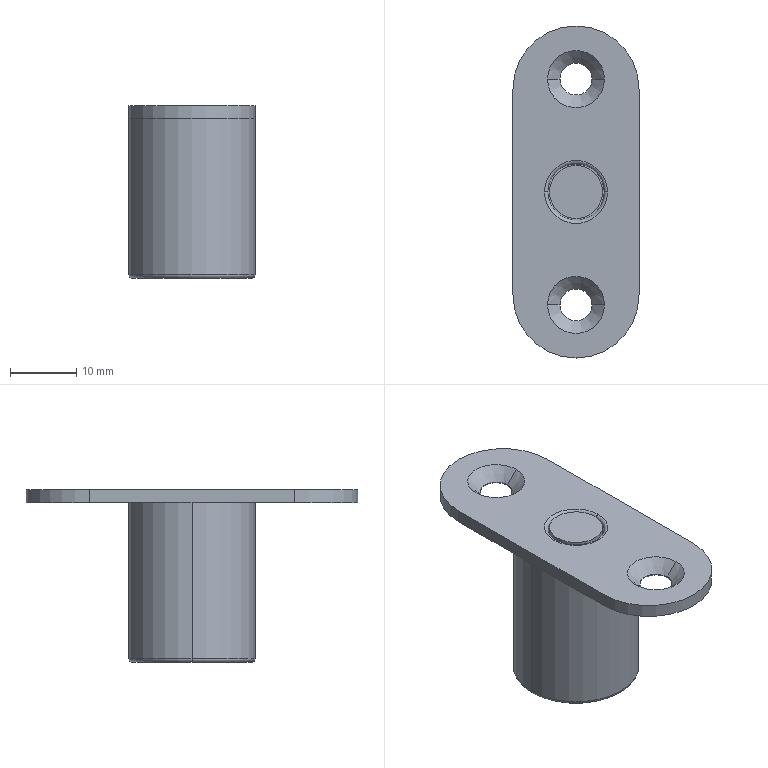Part | NX | features BREP 1 | 1 solid | 33 faces | box 19 x 50 x 26 mm | volume 8272 mm3 | plane 13 | cylinder 12 | cone 4 | torus 4 | commonest cylinder face diameters 4.8 x4 19 x4 8 x2 8.5 x2
STEP:
#1=CARTESIAN_POINT('',(-2.4,17.,-1.9));
#2=VERTEX_POINT('',#1);
#3=CARTESIAN_POINT('',(2.4,17.,-1.9));
#4=VERTEX_POINT('',#3);
#5=CARTESIAN_POINT('',(0.,17.,-1.9));
#6=DIRECTION('',(0.,0.,1.));
#7=DIRECTION('',(1.,0.,0.));
#8=AXIS2_PLACEMENT_3D('',#5,#6,#7);
#9=CIRCLE('',#8,2.4);
#10=EDGE_CURVE('',#2,#4,#9,.T.);
#11=ORIENTED_EDGE('',*,*,#10,.F.);
#12=CARTESIAN_POINT('',(-4.3,17.,0.));
#13=VERTEX_POINT('',#12);
#14=CARTESIAN_POINT('',(-2.4,17.,-1.9));
#15=DIRECTION('',(-0.7071,0.,0.7071));
#16=VECTOR('',#15,1000.);
#17=LINE('',#14,#16);
#18=EDGE_CURVE('',#13,#2,#17,.F.);
#19=ORIENTED_EDGE('',*,*,#18,.F.);
#20=CARTESIAN_POINT('',(4.3,17.,0.));
#21=VERTEX_POINT('',#20);
#22=CARTESIAN_POINT('',(0.,17.,0.));
#23=DIRECTION('',(0.,0.,-1.));
#24=DIRECTION('',(1.,0.,0.));
#25=AXIS2_PLACEMENT_3D('',#22,#23,#24);
#26=CIRCLE('',#25,4.3);
#27=EDGE_CURVE('',#21,#13,#26,.T.);
#28=ORIENTED_EDGE('',*,*,#27,.F.);
#29=CARTESIAN_POINT('',(2.4,17.,-1.9));
#30=DIRECTION('',(0.7071,0.,0.7071));
#31=VECTOR('',#30,1000.);
#32=LINE('',#29,#31);
#33=EDGE_CURVE('',#21,#4,#32,.F.);
#34=ORIENTED_EDGE('',*,*,#33,.T.);
#35=EDGE_LOOP('',(#11,#19,#28,#34));
#36=FACE_BOUND('',#35,.T.);
#37=CARTESIAN_POINT('',(0.,17.,-1.9));
#38=DIRECTION('',(0.,0.,1.));
#39=DIRECTION('',(1.,0.,0.));
#40=AXIS2_PLACEMENT_3D('',#37,#38,#39);
#41=CONICAL_SURFACE('',#40,2.4,0.7854);
#42=ADVANCED_FACE('',(#36),#41,.F.);
#43=CARTESIAN_POINT('',(-2.4,-17.,-1.9));
#44=VERTEX_POINT('',#43);
#45=CARTESIAN_POINT('',(2.4,-17.,-1.9));
#46=VERTEX_POINT('',#45);
#47=CARTESIAN_POINT('',(0.,-17.,-1.9));
#48=DIRECTION('',(0.,0.,1.));
#49=DIRECTION('',(1.,0.,0.));
#50=AXIS2_PLACEMENT_3D('',#47,#48,#49);
#51=CIRCLE('',#50,2.4);
#52=EDGE_CURVE('',#44,#46,#51,.T.);
#53=ORIENTED_EDGE('',*,*,#52,.F.);
#54=CARTESIAN_POINT('',(-4.3,-17.,0.));
#55=VERTEX_POINT('',#54);
#56=CARTESIAN_POINT('',(-2.4,-17.,-1.9));
#57=DIRECTION('',(-0.7071,0.,0.7071));
#58=VECTOR('',#57,1000.);
#59=LINE('',#56,#58);
#60=EDGE_CURVE('',#55,#44,#59,.F.);
#61=ORIENTED_EDGE('',*,*,#60,.F.);
#62=CARTESIAN_POINT('',(4.3,-17.,0.));
#63=VERTEX_POINT('',#62);
#64=CARTESIAN_POINT('',(0.,-17.,0.));
#65=DIRECTION('',(0.,0.,-1.));
#66=DIRECTION('',(1.,0.,0.));
#67=AXIS2_PLACEMENT_3D('',#64,#65,#66);
#68=CIRCLE('',#67,4.3);
#69=EDGE_CURVE('',#63,#55,#68,.T.);
#70=ORIENTED_EDGE('',*,*,#69,.F.);
#71=CARTESIAN_POINT('',(2.4,-17.,-1.9));
#72=DIRECTION('',(0.7071,0.,0.7071));
#73=VECTOR('',#72,1000.);
#74=LINE('',#71,#73);
#75=EDGE_CURVE('',#63,#46,#74,.F.);
#76=ORIENTED_EDGE('',*,*,#75,.T.);
#77=EDGE_LOOP('',(#53,#61,#70,#76));
#78=FACE_BOUND('',#77,.T.);
#79=CARTESIAN_POINT('',(0.,-17.,-1.9));
#80=DIRECTION('',(0.,0.,1.));
#81=DIRECTION('',(1.,0.,0.));
#82=AXIS2_PLACEMENT_3D('',#79,#80,#81);
#83=CONICAL_SURFACE('',#82,2.4,0.7854);
#84=ADVANCED_FACE('',(#78),#83,.F.);
#85=CARTESIAN_POINT('',(-4.75,0.,0.));
#86=VERTEX_POINT('',#85);
#87=CARTESIAN_POINT('',(4.75,0.,0.));
#88=VERTEX_POINT('',#87);
#89=CARTESIAN_POINT('',(0.,0.,0.));
#90=DIRECTION('',(0.,0.,-1.));
#91=DIRECTION('',(1.,0.,0.));
#92=AXIS2_PLACEMENT_3D('',#89,#90,#91);
#93=CIRCLE('',#92,4.75);
#94=EDGE_CURVE('',#86,#88,#93,.T.);
#95=ORIENTED_EDGE('',*,*,#94,.F.);
#96=CARTESIAN_POINT('',(-4.25,0.,-0.5));
#97=VERTEX_POINT('',#96);
#98=CARTESIAN_POINT('',(-4.75,0.,-0.5));
#99=DIRECTION('',(0.,1.,0.));
#100=DIRECTION('',(-1.,0.,0.));
#101=AXIS2_PLACEMENT_3D('',#98,#99,#100);
#102=CIRCLE('',#101,0.5);
#103=EDGE_CURVE('',#97,#86,#102,.F.);
#104=ORIENTED_EDGE('',*,*,#103,.F.);
#105=CARTESIAN_POINT('',(4.25,0.,-0.5));
#106=VERTEX_POINT('',#105);
#107=CARTESIAN_POINT('',(0.,0.,-0.5));
#108=DIRECTION('',(0.,0.,1.));
#109=DIRECTION('',(1.,0.,0.));
#110=AXIS2_PLACEMENT_3D('',#107,#108,#109);
#111=CIRCLE('',#110,4.25);
#112=EDGE_CURVE('',#106,#97,#111,.T.);
#113=ORIENTED_EDGE('',*,*,#112,.F.);
#114=CARTESIAN_POINT('',(4.75,0.,-0.5));
#115=DIRECTION('',(0.,-1.,0.));
#116=DIRECTION('',(0.,0.,-1.));
#117=AXIS2_PLACEMENT_3D('',#114,#115,#116);
#118=CIRCLE('',#117,0.5);
#119=EDGE_CURVE('',#106,#88,#118,.F.);
#120=ORIENTED_EDGE('',*,*,#119,.T.);
#121=EDGE_LOOP('',(#95,#104,#113,#120));
#122=FACE_BOUND('',#121,.T.);
#123=CARTESIAN_POINT('',(0.,0.,-0.5));
#124=DIRECTION('',(0.,0.,1.));
#125=DIRECTION('',(1.,0.,0.));
#126=AXIS2_PLACEMENT_3D('',#123,#124,#125);
#127=TOROIDAL_SURFACE('',#126,4.75,0.5);
#128=ADVANCED_FACE('',(#122),#127,.T.);
#129=CARTESIAN_POINT('',(9.5,0.,-25.5));
#130=VERTEX_POINT('',#129);
#131=CARTESIAN_POINT('',(-9.5,0.,-25.5));
#132=VERTEX_POINT('',#131);
#133=CARTESIAN_POINT('',(0.,0.,-25.5));
#134=DIRECTION('',(0.,0.,1.));
#135=DIRECTION('',(-1.,0.,0.));
#136=AXIS2_PLACEMENT_3D('',#133,#134,#135);
#137=CIRCLE('',#136,9.5);
#138=EDGE_CURVE('',#130,#132,#137,.T.);
#139=ORIENTED_EDGE('',*,*,#138,.F.);
#140=CARTESIAN_POINT('',(9.,0.,-26.));
#141=VERTEX_POINT('',#140);
#142=CARTESIAN_POINT('',(9.,0.,-25.5));
#143=DIRECTION('',(0.,1.,0.));
#144=DIRECTION('',(-1.,0.,0.));
#145=AXIS2_PLACEMENT_3D('',#142,#143,#144);
#146=CIRCLE('',#145,0.5);
#147=EDGE_CURVE('',#130,#141,#146,.T.);
#148=ORIENTED_EDGE('',*,*,#147,.T.);
#149=CARTESIAN_POINT('',(-9.,0.,-26.));
#150=VERTEX_POINT('',#149);
#151=CARTESIAN_POINT('',(0.,0.,-26.));
#152=DIRECTION('',(0.,0.,-1.));
#153=DIRECTION('',(-1.,0.,0.));
#154=AXIS2_PLACEMENT_3D('',#151,#152,#153);
#155=CIRCLE('',#154,9.);
#156=EDGE_CURVE('',#150,#141,#155,.T.);
#157=ORIENTED_EDGE('',*,*,#156,.F.);
#158=CARTESIAN_POINT('',(-9.,0.,-25.5));
#159=DIRECTION('',(0.,-1.,0.));
#160=DIRECTION('',(0.,0.,-1.));
#161=AXIS2_PLACEMENT_3D('',#158,#159,#160);
#162=CIRCLE('',#161,0.5);
#163=EDGE_CURVE('',#132,#150,#162,.T.);
#164=ORIENTED_EDGE('',*,*,#163,.F.);
#165=EDGE_LOOP('',(#139,#148,#157,#164));
#166=FACE_BOUND('',#165,.T.);
#167=CARTESIAN_POINT('',(0.,0.,-25.5));
#168=DIRECTION('',(0.,0.,-1.));
#169=DIRECTION('',(-1.,0.,0.));
#170=AXIS2_PLACEMENT_3D('',#167,#168,#169);
#171=TOROIDAL_SURFACE('',#170,9.,0.5);
#172=ADVANCED_FACE('',(#166),#171,.T.);
#173=CARTESIAN_POINT('',(4.,0.,-5.));
#174=VERTEX_POINT('',#173);
#175=CARTESIAN_POINT('',(-4.,0.,-5.));
#176=VERTEX_POINT('',#175);
#177=CARTESIAN_POINT('',(0.,0.,-5.));
#178=DIRECTION('',(0.,0.,1.));
#179=DIRECTION('',(1.,0.,0.));
#180=AXIS2_PLACEMENT_3D('',#177,#178,#179);
#181=CIRCLE('',#180,4.);
#182=EDGE_CURVE('',#174,#176,#181,.T.);
#183=ORIENTED_EDGE('',*,*,#182,.T.);
#184=CARTESIAN_POINT('',(-4.,0.,0.));
#185=VERTEX_POINT('',#184);
#186=CARTESIAN_POINT('',(-4.,0.,-5.));
#187=DIRECTION('',(0.,0.,1.));
#188=VECTOR('',#187,1000.);
#189=LINE('',#186,#188);
#190=EDGE_CURVE('',#185,#176,#189,.F.);
#191=ORIENTED_EDGE('',*,*,#190,.F.);
#192=CARTESIAN_POINT('',(4.,0.,0.));
#193=VERTEX_POINT('',#192);
#194=CARTESIAN_POINT('',(0.,0.,0.));
#195=DIRECTION('',(0.,0.,1.));
#196=DIRECTION('',(1.,0.,0.));
#197=AXIS2_PLACEMENT_3D('',#194,#195,#196);
#198=CIRCLE('',#197,4.);
#199=EDGE_CURVE('',#193,#185,#198,.T.);
#200=ORIENTED_EDGE('',*,*,#199,.F.);
#201=CARTESIAN_POINT('',(4.,0.,-5.));
#202=DIRECTION('',(0.,0.,1.));
#203=VECTOR('',#202,1000.);
#204=LINE('',#201,#203);
#205=EDGE_CURVE('',#193,#174,#204,.F.);
#206=ORIENTED_EDGE('',*,*,#205,.T.);
#207=EDGE_LOOP('',(#183,#191,#200,#206));
#208=FACE_BOUND('',#207,.T.);
#209=CARTESIAN_POINT('',(0.,0.,-5.));
#210=DIRECTION('',(0.,0.,1.));
#211=DIRECTION('',(1.,0.,0.));
#212=AXIS2_PLACEMENT_3D('',#209,#210,#211);
#213=CYLINDRICAL_SURFACE('',#212,4.);
#214=ADVANCED_FACE('',(#208),#213,.T.);
#215=CARTESIAN_POINT('',(-4.25,0.,-5.));
#216=VERTEX_POINT('',#215);
#217=CARTESIAN_POINT('',(4.25,0.,-5.));
#218=VERTEX_POINT('',#217);
#219=CARTESIAN_POINT('',(0.,0.,-5.));
#220=DIRECTION('',(0.,0.,1.));
#221=DIRECTION('',(1.,0.,0.));
#222=AXIS2_PLACEMENT_3D('',#219,#220,#221);
#223=CIRCLE('',#222,4.25);
#224=EDGE_CURVE('',#216,#218,#223,.T.);
#225=ORIENTED_EDGE('',*,*,#224,.F.);
#226=CARTESIAN_POINT('',(-4.25,0.,-5.));
#227=DIRECTION('',(0.,0.,1.));
#228=VECTOR('',#227,1000.);
#229=LINE('',#226,#228);
#230=EDGE_CURVE('',#97,#216,#229,.F.);
#231=ORIENTED_EDGE('',*,*,#230,.F.);
#232=CARTESIAN_POINT('',(0.,0.,-0.5));
#233=DIRECTION('',(0.,0.,1.));
#234=DIRECTION('',(1.,0.,0.));
#235=AXIS2_PLACEMENT_3D('',#232,#233,#234);
#236=CIRCLE('',#235,4.25);
#237=EDGE_CURVE('',#97,#106,#236,.T.);
#238=ORIENTED_EDGE('',*,*,#237,.T.);
#239=CARTESIAN_POINT('',(4.25,0.,-5.));
#240=DIRECTION('',(0.,0.,1.));
#241=VECTOR('',#240,1000.);
#242=LINE('',#239,#241);
#243=EDGE_CURVE('',#106,#218,#242,.F.);
#244=ORIENTED_EDGE('',*,*,#243,.T.);
#245=EDGE_LOOP('',(#225,#231,#238,#244));
#246=FACE_BOUND('',#245,.T.);
#247=CARTESIAN_POINT('',(0.,0.,-5.));
#248=DIRECTION('',(0.,0.,1.));
#249=DIRECTION('',(1.,0.,0.));
#250=AXIS2_PLACEMENT_3D('',#247,#248,#249);
#251=CYLINDRICAL_SURFACE('',#250,4.25);
#252=ADVANCED_FACE('',(#246),#251,.F.);
#253=ORIENTED_EDGE('',*,*,#138,.T.);
#254=CARTESIAN_POINT('',(-9.5,0.,-2.));
#255=VERTEX_POINT('',#254);
#256=CARTESIAN_POINT('',(-9.5,0.,-26.));
#257=DIRECTION('',(0.,0.,1.));
#258=VECTOR('',#257,1000.);
#259=LINE('',#256,#258);
#260=EDGE_CURVE('',#255,#132,#259,.F.);
#261=ORIENTED_EDGE('',*,*,#260,.F.);
#262=CARTESIAN_POINT('',(9.5,0.,-2.));
#263=VERTEX_POINT('',#262);
#264=CARTESIAN_POINT('',(0.,0.,-2.));
#265=DIRECTION('',(0.,0.,-1.));
#266=DIRECTION('',(-1.,0.,0.));
#267=AXIS2_PLACEMENT_3D('',#264,#265,#266);
#268=CIRCLE('',#267,9.5);
#269=EDGE_CURVE('',#255,#263,#268,.T.);
#270=ORIENTED_EDGE('',*,*,#269,.T.);
#271=CARTESIAN_POINT('',(9.5,0.,-26.));
#272=DIRECTION('',(0.,0.,1.));
#273=VECTOR('',#272,1000.);
#274=LINE('',#271,#273);
#275=EDGE_CURVE('',#263,#130,#274,.F.);
#276=ORIENTED_EDGE('',*,*,#275,.T.);
#277=EDGE_LOOP('',(#253,#261,#270,#276));
#278=FACE_BOUND('',#277,.T.);
#279=CARTESIAN_POINT('',(0.,0.,-26.));
#280=DIRECTION('',(0.,0.,1.));
#281=DIRECTION('',(1.,0.,0.));
#282=AXIS2_PLACEMENT_3D('',#279,#280,#281);
#283=CYLINDRICAL_SURFACE('',#282,9.5);
#284=ADVANCED_FACE('',(#278),#283,.T.);
#285=CARTESIAN_POINT('',(-2.4,-17.,-2.));
#286=VERTEX_POINT('',#285);
#287=CARTESIAN_POINT('',(2.4,-17.,-2.));
#288=VERTEX_POINT('',#287);
#289=CARTESIAN_POINT('',(0.,-17.,-2.));
#290=DIRECTION('',(0.,0.,1.));
#291=DIRECTION('',(1.,0.,0.));
#292=AXIS2_PLACEMENT_3D('',#289,#290,#291);
#293=CIRCLE('',#292,2.4);
#294=EDGE_CURVE('',#286,#288,#293,.T.);
#295=ORIENTED_EDGE('',*,*,#294,.F.);
#296=CARTESIAN_POINT('',(-2.4,-17.,-2.));
#297=DIRECTION('',(0.,0.,1.));
#298=VECTOR('',#297,1000.);
#299=LINE('',#296,#298);
#300=EDGE_CURVE('',#44,#286,#299,.F.);
#301=ORIENTED_EDGE('',*,*,#300,.F.);
#302=ORIENTED_EDGE('',*,*,#52,.T.);
#303=CARTESIAN_POINT('',(2.4,-17.,-2.));
#304=DIRECTION('',(0.,0.,1.));
#305=VECTOR('',#304,1000.);
#306=LINE('',#303,#305);
#307=EDGE_CURVE('',#46,#288,#306,.F.);
#308=ORIENTED_EDGE('',*,*,#307,.T.);
#309=EDGE_LOOP('',(#295,#301,#302,#308));
#310=FACE_BOUND('',#309,.T.);
#311=CARTESIAN_POINT('',(0.,-17.,-2.));
#312=DIRECTION('',(0.,0.,1.));
#313=DIRECTION('',(1.,0.,0.));
#314=AXIS2_PLACEMENT_3D('',#311,#312,#313);
#315=CYLINDRICAL_SURFACE('',#314,2.4);
#316=ADVANCED_FACE('',(#310),#315,.F.);
#317=CARTESIAN_POINT('',(-2.4,17.,-2.));
#318=VERTEX_POINT('',#317);
#319=CARTESIAN_POINT('',(2.4,17.,-2.));
#320=VERTEX_POINT('',#319);
#321=CARTESIAN_POINT('',(0.,17.,-2.));
#322=DIRECTION('',(0.,0.,1.));
#323=DIRECTION('',(1.,0.,0.));
#324=AXIS2_PLACEMENT_3D('',#321,#322,#323);
#325=CIRCLE('',#324,2.4);
#326=EDGE_CURVE('',#318,#320,#325,.T.);
#327=ORIENTED_EDGE('',*,*,#326,.F.);
#328=CARTESIAN_POINT('',(-2.4,17.,-2.));
#329=DIRECTION('',(0.,0.,1.));
#330=VECTOR('',#329,1000.);
#331=LINE('',#328,#330);
#332=EDGE_CURVE('',#2,#318,#331,.F.);
#333=ORIENTED_EDGE('',*,*,#332,.F.);
#334=ORIENTED_EDGE('',*,*,#10,.T.);
#335=CARTESIAN_POINT('',(2.4,17.,-2.));
#336=DIRECTION('',(0.,0.,1.));
#337=VECTOR('',#336,1000.);
#338=LINE('',#335,#337);
#339=EDGE_CURVE('',#4,#320,#338,.F.);
#340=ORIENTED_EDGE('',*,*,#339,.T.);
#341=EDGE_LOOP('',(#327,#333,#334,#340));
#342=FACE_BOUND('',#341,.T.);
#343=CARTESIAN_POINT('',(0.,17.,-2.));
#344=DIRECTION('',(0.,0.,1.));
#345=DIRECTION('',(1.,0.,0.));
#346=AXIS2_PLACEMENT_3D('',#343,#344,#345);
#347=CYLINDRICAL_SURFACE('',#346,2.4);
#348=ADVANCED_FACE('',(#342),#347,.F.);
#349=ORIENTED_EDGE('',*,*,#269,.F.);
#350=CARTESIAN_POINT('',(-9.5,15.5,-2.));
#351=VERTEX_POINT('',#350);
#352=CARTESIAN_POINT('',(-9.5,15.5,-2.));
#353=DIRECTION('',(0.,-1.,0.));
#354=VECTOR('',#353,1000.);
#355=LINE('',#352,#354);
#356=EDGE_CURVE('',#351,#255,#355,.T.);
#357=ORIENTED_EDGE('',*,*,#356,.F.);
#358=CARTESIAN_POINT('',(9.5,15.5,-2.));
#359=VERTEX_POINT('',#358);
#360=CARTESIAN_POINT('',(0.,15.5,-2.));
#361=DIRECTION('',(0.,0.,1.));
#362=DIRECTION('',(1.,0.,0.));
#363=AXIS2_PLACEMENT_3D('',#360,#361,#362);
#364=CIRCLE('',#363,9.5);
#365=EDGE_CURVE('',#359,#351,#364,.T.);
#366=ORIENTED_EDGE('',*,*,#365,.F.);
#367=CARTESIAN_POINT('',(9.5,15.5,-2.));
#368=DIRECTION('',(0.,1.,0.));
#369=VECTOR('',#368,1000.);
#370=LINE('',#367,#369);
#371=EDGE_CURVE('',#263,#359,#370,.T.);
#372=ORIENTED_EDGE('',*,*,#371,.F.);
#373=EDGE_LOOP('',(#349,#357,#366,#372));
#374=FACE_BOUND('',#373,.T.);
#375=CARTESIAN_POINT('',(0.,17.,-2.));
#376=DIRECTION('',(0.,0.,1.));
#377=DIRECTION('',(1.,0.,0.));
#378=AXIS2_PLACEMENT_3D('',#375,#376,#377);
#379=CIRCLE('',#378,2.4);
#380=EDGE_CURVE('',#320,#318,#379,.T.);
#381=ORIENTED_EDGE('',*,*,#380,.T.);
#382=ORIENTED_EDGE('',*,*,#326,.T.);
#383=EDGE_LOOP('',(#381,#382));
#384=FACE_BOUND('',#383,.T.);
#385=CARTESIAN_POINT('',(0.,15.5,-2.));
#386=DIRECTION('',(0.,0.,1.));
#387=DIRECTION('',(1.,0.,0.));
#388=AXIS2_PLACEMENT_3D('',#385,#386,#387);
#389=PLANE('',#388);
#390=ADVANCED_FACE('',(#374,#384),#389,.F.);
#391=CARTESIAN_POINT('',(0.,0.,-2.));
#392=DIRECTION('',(0.,0.,-1.));
#393=DIRECTION('',(-1.,0.,0.));
#394=AXIS2_PLACEMENT_3D('',#391,#392,#393);
#395=CIRCLE('',#394,9.5);
#396=EDGE_CURVE('',#263,#255,#395,.T.);
#397=ORIENTED_EDGE('',*,*,#396,.F.);
#398=CARTESIAN_POINT('',(9.5,-15.5,-2.));
#399=VERTEX_POINT('',#398);
#400=CARTESIAN_POINT('',(9.5,15.5,-2.));
#401=DIRECTION('',(0.,1.,0.));
#402=VECTOR('',#401,1000.);
#403=LINE('',#400,#402);
#404=EDGE_CURVE('',#399,#263,#403,.T.);
#405=ORIENTED_EDGE('',*,*,#404,.F.);
#406=CARTESIAN_POINT('',(-9.5,-15.5,-2.));
#407=VERTEX_POINT('',#406);
#408=CARTESIAN_POINT('',(0.,-15.5,-2.));
#409=DIRECTION('',(0.,0.,1.));
#410=DIRECTION('',(1.,0.,0.));
#411=AXIS2_PLACEMENT_3D('',#408,#409,#410);
#412=CIRCLE('',#411,9.5);
#413=EDGE_CURVE('',#407,#399,#412,.T.);
#414=ORIENTED_EDGE('',*,*,#413,.F.);
#415=CARTESIAN_POINT('',(-9.5,15.5,-2.));
#416=DIRECTION('',(0.,-1.,0.));
#417=VECTOR('',#416,1000.);
#418=LINE('',#415,#417);
#419=EDGE_CURVE('',#255,#407,#418,.T.);
#420=ORIENTED_EDGE('',*,*,#419,.F.);
#421=EDGE_LOOP('',(#397,#405,#414,#420));
#422=FACE_BOUND('',#421,.T.);
#423=CARTESIAN_POINT('',(0.,-17.,-2.));
#424=DIRECTION('',(0.,0.,1.));
#425=DIRECTION('',(1.,0.,0.));
#426=AXIS2_PLACEMENT_3D('',#423,#424,#425);
#427=CIRCLE('',#426,2.4);
#428=EDGE_CURVE('',#288,#286,#427,.T.);
#429=ORIENTED_EDGE('',*,*,#428,.T.);
#430=ORIENTED_EDGE('',*,*,#294,.T.);
#431=EDGE_LOOP('',(#429,#430));
#432=FACE_BOUND('',#431,.T.);
#433=CARTESIAN_POINT('',(0.,15.5,-2.));
#434=DIRECTION('',(0.,0.,1.));
#435=DIRECTION('',(1.,0.,0.));
#436=AXIS2_PLACEMENT_3D('',#433,#434,#435);
#437=PLANE('',#436);
#438=ADVANCED_FACE('',(#422,#432),#437,.F.);
#439=CARTESIAN_POINT('',(9.5,15.5,0.));
#440=VERTEX_POINT('',#439);
#441=CARTESIAN_POINT('',(-9.5,15.5,0.));
#442=VERTEX_POINT('',#441);
#443=CARTESIAN_POINT('',(0.,15.5,0.));
#444=DIRECTION('',(0.,0.,1.));
#445=DIRECTION('',(1.,0.,0.));
#446=AXIS2_PLACEMENT_3D('',#443,#444,#445);
#447=CIRCLE('',#446,9.5);
#448=EDGE_CURVE('',#440,#442,#447,.T.);
#449=ORIENTED_EDGE('',*,*,#448,.F.);
#450=CARTESIAN_POINT('',(9.5,15.5,-2.));
#451=DIRECTION('',(0.,0.,1.));
#452=VECTOR('',#451,1000.);
#453=LINE('',#450,#452);
#454=EDGE_CURVE('',#359,#440,#453,.T.);
#455=ORIENTED_EDGE('',*,*,#454,.F.);
#456=ORIENTED_EDGE('',*,*,#365,.T.);
#457=CARTESIAN_POINT('',(-9.5,15.5,-2.));
#458=DIRECTION('',(0.,0.,1.));
#459=VECTOR('',#458,1000.);
#460=LINE('',#457,#459);
#461=EDGE_CURVE('',#351,#442,#460,.T.);
#462=ORIENTED_EDGE('',*,*,#461,.T.);
#463=EDGE_LOOP('',(#449,#455,#456,#462));
#464=FACE_BOUND('',#463,.T.);
#465=CARTESIAN_POINT('',(0.,15.5,-2.));
#466=DIRECTION('',(0.,0.,1.));
#467=DIRECTION('',(1.,0.,0.));
#468=AXIS2_PLACEMENT_3D('',#465,#466,#467);
#469=CYLINDRICAL_SURFACE('',#468,9.5);
#470=ADVANCED_FACE('',(#464),#469,.T.);
#471=CARTESIAN_POINT('',(9.5,-15.5,0.));
#472=VERTEX_POINT('',#471);
#473=CARTESIAN_POINT('',(9.5,15.5,0.));
#474=DIRECTION('',(0.,1.,0.));
#475=VECTOR('',#474,1000.);
#476=LINE('',#473,#475);
#477=EDGE_CURVE('',#472,#440,#476,.T.);
#478=ORIENTED_EDGE('',*,*,#477,.F.);
#479=CARTESIAN_POINT('',(9.5,-15.5,-2.));
#480=DIRECTION('',(0.,0.,1.));
#481=VECTOR('',#480,1000.);
#482=LINE('',#479,#481);
#483=EDGE_CURVE('',#399,#472,#482,.T.);
#484=ORIENTED_EDGE('',*,*,#483,.F.);
#485=ORIENTED_EDGE('',*,*,#404,.T.);
#486=ORIENTED_EDGE('',*,*,#371,.T.);
#487=ORIENTED_EDGE('',*,*,#454,.T.);
#488=EDGE_LOOP('',(#478,#484,#485,#486,#487));
#489=FACE_BOUND('',#488,.T.);
#490=CARTESIAN_POINT('',(9.5,15.5,-2.));
#491=DIRECTION('',(1.,0.,0.));
#492=DIRECTION('',(0.,1.,0.));
#493=AXIS2_PLACEMENT_3D('',#490,#491,#492);
#494=PLANE('',#493);
#495=ADVANCED_FACE('',(#489),#494,.T.);
#496=CARTESIAN_POINT('',(-9.5,-15.5,0.));
#497=VERTEX_POINT('',#496);
#498=CARTESIAN_POINT('',(0.,-15.5,0.));
#499=DIRECTION('',(0.,0.,1.));
#500=DIRECTION('',(1.,0.,0.));
#501=AXIS2_PLACEMENT_3D('',#498,#499,#500);
#502=CIRCLE('',#501,9.5);
#503=EDGE_CURVE('',#497,#472,#502,.T.);
#504=ORIENTED_EDGE('',*,*,#503,.F.);
#505=CARTESIAN_POINT('',(-9.5,-15.5,-2.));
#506=DIRECTION('',(0.,0.,1.));
#507=VECTOR('',#506,1000.);
#508=LINE('',#505,#507);
#509=EDGE_CURVE('',#407,#497,#508,.T.);
#510=ORIENTED_EDGE('',*,*,#509,.F.);
#511=ORIENTED_EDGE('',*,*,#413,.T.);
#512=ORIENTED_EDGE('',*,*,#483,.T.);
#513=EDGE_LOOP('',(#504,#510,#511,#512));
#514=FACE_BOUND('',#513,.T.);
#515=CARTESIAN_POINT('',(0.,-15.5,-2.));
#516=DIRECTION('',(0.,0.,1.));
#517=DIRECTION('',(1.,0.,0.));
#518=AXIS2_PLACEMENT_3D('',#515,#516,#517);
#519=CYLINDRICAL_SURFACE('',#518,9.5);
#520=ADVANCED_FACE('',(#514),#519,.T.);
#521=CARTESIAN_POINT('',(-9.5,15.5,0.));
#522=DIRECTION('',(0.,-1.,0.));
#523=VECTOR('',#522,1000.);
#524=LINE('',#521,#523);
#525=EDGE_CURVE('',#442,#497,#524,.T.);
#526=ORIENTED_EDGE('',*,*,#525,.F.);
#527=ORIENTED_EDGE('',*,*,#461,.F.);
#528=ORIENTED_EDGE('',*,*,#356,.T.);
#529=ORIENTED_EDGE('',*,*,#419,.T.);
#530=ORIENTED_EDGE('',*,*,#509,.T.);
#531=EDGE_LOOP('',(#526,#527,#528,#529,#530));
#532=FACE_BOUND('',#531,.T.);
#533=CARTESIAN_POINT('',(-9.5,15.5,-2.));
#534=DIRECTION('',(-1.,0.,0.));
#535=DIRECTION('',(0.,1.,0.));
#536=AXIS2_PLACEMENT_3D('',#533,#534,#535);
#537=PLANE('',#536);
#538=ADVANCED_FACE('',(#532),#537,.T.);
#539=ORIENTED_EDGE('',*,*,#448,.T.);
#540=ORIENTED_EDGE('',*,*,#525,.T.);
#541=ORIENTED_EDGE('',*,*,#503,.T.);
#542=ORIENTED_EDGE('',*,*,#477,.T.);
#543=EDGE_LOOP('',(#539,#540,#541,#542));
#544=FACE_BOUND('',#543,.T.);
#545=ORIENTED_EDGE('',*,*,#69,.T.);
#546=CARTESIAN_POINT('',(0.,-17.,0.));
#547=DIRECTION('',(0.,0.,-1.));
#548=DIRECTION('',(1.,0.,0.));
#549=AXIS2_PLACEMENT_3D('',#546,#547,#548);
#550=CIRCLE('',#549,4.3);
#551=EDGE_CURVE('',#55,#63,#550,.T.);
#552=ORIENTED_EDGE('',*,*,#551,.T.);
#553=EDGE_LOOP('',(#545,#552));
#554=FACE_BOUND('',#553,.T.);
#555=ORIENTED_EDGE('',*,*,#27,.T.);
#556=CARTESIAN_POINT('',(0.,17.,0.));
#557=DIRECTION('',(0.,0.,-1.));
#558=DIRECTION('',(1.,0.,0.));
#559=AXIS2_PLACEMENT_3D('',#556,#557,#558);
#560=CIRCLE('',#559,4.3);
#561=EDGE_CURVE('',#13,#21,#560,.T.);
#562=ORIENTED_EDGE('',*,*,#561,.T.);
#563=EDGE_LOOP('',(#555,#562));
#564=FACE_BOUND('',#563,.T.);
#565=CARTESIAN_POINT('',(0.,0.,0.));
#566=DIRECTION('',(0.,0.,-1.));
#567=DIRECTION('',(1.,0.,0.));
#568=AXIS2_PLACEMENT_3D('',#565,#566,#567);
#569=CIRCLE('',#568,4.75);
#570=EDGE_CURVE('',#88,#86,#569,.T.);
#571=ORIENTED_EDGE('',*,*,#570,.T.);
#572=ORIENTED_EDGE('',*,*,#94,.T.);
#573=EDGE_LOOP('',(#571,#572));
#574=FACE_BOUND('',#573,.T.);
#575=CARTESIAN_POINT('',(0.,15.5,0.));
#576=DIRECTION('',(0.,0.,1.));
#577=DIRECTION('',(1.,0.,0.));
#578=AXIS2_PLACEMENT_3D('',#575,#576,#577);
#579=PLANE('',#578);
#580=ADVANCED_FACE('',(#544,#554,#564,#574),#579,.T.);
#581=ORIENTED_EDGE('',*,*,#332,.T.);
#582=ORIENTED_EDGE('',*,*,#380,.F.);
#583=ORIENTED_EDGE('',*,*,#339,.F.);
#584=CARTESIAN_POINT('',(0.,17.,-1.9));
#585=DIRECTION('',(0.,0.,1.));
#586=DIRECTION('',(1.,0.,0.));
#587=AXIS2_PLACEMENT_3D('',#584,#585,#586);
#588=CIRCLE('',#587,2.4);
#589=EDGE_CURVE('',#4,#2,#588,.T.);
#590=ORIENTED_EDGE('',*,*,#589,.T.);
#591=EDGE_LOOP('',(#581,#582,#583,#590));
#592=FACE_BOUND('',#591,.T.);
#593=CARTESIAN_POINT('',(0.,17.,-2.));
#594=DIRECTION('',(0.,0.,1.));
#595=DIRECTION('',(1.,0.,0.));
#596=AXIS2_PLACEMENT_3D('',#593,#594,#595);
#597=CYLINDRICAL_SURFACE('',#596,2.4);
#598=ADVANCED_FACE('',(#592),#597,.F.);
#599=ORIENTED_EDGE('',*,*,#300,.T.);
#600=ORIENTED_EDGE('',*,*,#428,.F.);
#601=ORIENTED_EDGE('',*,*,#307,.F.);
#602=CARTESIAN_POINT('',(0.,-17.,-1.9));
#603=DIRECTION('',(0.,0.,1.));
#604=DIRECTION('',(1.,0.,0.));
#605=AXIS2_PLACEMENT_3D('',#602,#603,#604);
#606=CIRCLE('',#605,2.4);
#607=EDGE_CURVE('',#46,#44,#606,.T.);
#608=ORIENTED_EDGE('',*,*,#607,.T.);
#609=EDGE_LOOP('',(#599,#600,#601,#608));
#610=FACE_BOUND('',#609,.T.);
#611=CARTESIAN_POINT('',(0.,-17.,-2.));
#612=DIRECTION('',(0.,0.,1.));
#613=DIRECTION('',(1.,0.,0.));
#614=AXIS2_PLACEMENT_3D('',#611,#612,#613);
#615=CYLINDRICAL_SURFACE('',#614,2.4);
#616=ADVANCED_FACE('',(#610),#615,.F.);
#617=ORIENTED_EDGE('',*,*,#260,.T.);
#618=CARTESIAN_POINT('',(0.,0.,-25.5));
#619=DIRECTION('',(0.,0.,1.));
#620=DIRECTION('',(-1.,0.,0.));
#621=AXIS2_PLACEMENT_3D('',#618,#619,#620);
#622=CIRCLE('',#621,9.5);
#623=EDGE_CURVE('',#132,#130,#622,.T.);
#624=ORIENTED_EDGE('',*,*,#623,.T.);
#625=ORIENTED_EDGE('',*,*,#275,.F.);
#626=ORIENTED_EDGE('',*,*,#396,.T.);
#627=EDGE_LOOP('',(#617,#624,#625,#626));
#628=FACE_BOUND('',#627,.T.);
#629=CARTESIAN_POINT('',(0.,0.,-26.));
#630=DIRECTION('',(0.,0.,1.));
#631=DIRECTION('',(1.,0.,0.));
#632=AXIS2_PLACEMENT_3D('',#629,#630,#631);
#633=CYLINDRICAL_SURFACE('',#632,9.5);
#634=ADVANCED_FACE('',(#628),#633,.T.);
#635=ORIENTED_EDGE('',*,*,#156,.T.);
#636=CARTESIAN_POINT('',(0.,0.,-26.));
#637=DIRECTION('',(0.,0.,-1.));
#638=DIRECTION('',(-1.,0.,0.));
#639=AXIS2_PLACEMENT_3D('',#636,#637,#638);
#640=CIRCLE('',#639,9.);
#641=EDGE_CURVE('',#141,#150,#640,.T.);
#642=ORIENTED_EDGE('',*,*,#641,.T.);
#643=EDGE_LOOP('',(#635,#642));
#644=FACE_BOUND('',#643,.T.);
#645=CARTESIAN_POINT('',(-1.,-5.,-26.));
#646=VERTEX_POINT('',#645);
#647=CARTESIAN_POINT('',(-1.,5.,-26.));
#648=VERTEX_POINT('',#647);
#649=CARTESIAN_POINT('',(-1.,-5.,-26.));
#650=DIRECTION('',(0.,1.,0.));
#651=VECTOR('',#650,1000.);
#652=LINE('',#649,#651);
#653=EDGE_CURVE('',#646,#648,#652,.T.);
#654=ORIENTED_EDGE('',*,*,#653,.F.);
#655=CARTESIAN_POINT('',(1.,-5.,-26.));
#656=VERTEX_POINT('',#655);
#657=CARTESIAN_POINT('',(1.,-5.,-26.));
#658=DIRECTION('',(-1.,0.,0.));
#659=VECTOR('',#658,1000.);
#660=LINE('',#657,#659);
#661=EDGE_CURVE('',#656,#646,#660,.T.);
#662=ORIENTED_EDGE('',*,*,#661,.F.);
#663=CARTESIAN_POINT('',(1.,5.,-26.));
#664=VERTEX_POINT('',#663);
#665=CARTESIAN_POINT('',(1.,-5.,-26.));
#666=DIRECTION('',(0.,-1.,0.));
#667=VECTOR('',#666,1000.);
#668=LINE('',#665,#667);
#669=EDGE_CURVE('',#664,#656,#668,.T.);
#670=ORIENTED_EDGE('',*,*,#669,.F.);
#671=CARTESIAN_POINT('',(1.,5.,-26.));
#672=DIRECTION('',(1.,0.,0.));
#673=VECTOR('',#672,1000.);
#674=LINE('',#671,#673);
#675=EDGE_CURVE('',#648,#664,#674,.T.);
#676=ORIENTED_EDGE('',*,*,#675,.F.);
#677=EDGE_LOOP('',(#654,#662,#670,#676));
#678=FACE_BOUND('',#677,.T.);
#679=CARTESIAN_POINT('',(0.,0.,-26.));
#680=DIRECTION('',(0.,0.,-1.));
#681=DIRECTION('',(0.,-1.,0.));
#682=AXIS2_PLACEMENT_3D('',#679,#680,#681);
#683=PLANE('',#682);
#684=ADVANCED_FACE('',(#644,#678),#683,.T.);
#685=ORIENTED_EDGE('',*,*,#653,.T.);
#686=CARTESIAN_POINT('',(-1.,5.,-21.));
#687=VERTEX_POINT('',#686);
#688=CARTESIAN_POINT('',(-1.,5.,-21.));
#689=DIRECTION('',(0.,0.,-1.));
#690=VECTOR('',#689,1000.);
#691=LINE('',#688,#690);
#692=EDGE_CURVE('',#687,#648,#691,.T.);
#693=ORIENTED_EDGE('',*,*,#692,.F.);
#694=CARTESIAN_POINT('',(-1.,-5.,-21.));
#695=VERTEX_POINT('',#694);
#696=CARTESIAN_POINT('',(-1.,-5.,-21.));
#697=DIRECTION('',(0.,1.,0.));
#698=VECTOR('',#697,1000.);
#699=LINE('',#696,#698);
#700=EDGE_CURVE('',#695,#687,#699,.T.);
#701=ORIENTED_EDGE('',*,*,#700,.F.);
#702=CARTESIAN_POINT('',(-1.,-5.,-21.));
#703=DIRECTION('',(0.,0.,-1.));
#704=VECTOR('',#703,1000.);
#705=LINE('',#702,#704);
#706=EDGE_CURVE('',#695,#646,#705,.T.);
#707=ORIENTED_EDGE('',*,*,#706,.T.);
#708=EDGE_LOOP('',(#685,#693,#701,#707));
#709=FACE_BOUND('',#708,.T.);
#710=CARTESIAN_POINT('',(-1.,-5.,-21.));
#711=DIRECTION('',(-1.,0.,0.));
#712=DIRECTION('',(0.,0.,1.));
#713=AXIS2_PLACEMENT_3D('',#710,#711,#712);
#714=PLANE('',#713);
#715=ADVANCED_FACE('',(#709),#714,.F.);
#716=ORIENTED_EDGE('',*,*,#661,.T.);
#717=ORIENTED_EDGE('',*,*,#706,.F.);
#718=CARTESIAN_POINT('',(1.,-5.,-21.));
#719=VERTEX_POINT('',#718);
#720=CARTESIAN_POINT('',(1.,-5.,-21.));
#721=DIRECTION('',(-1.,0.,0.));
#722=VECTOR('',#721,1000.);
#723=LINE('',#720,#722);
#724=EDGE_CURVE('',#719,#695,#723,.T.);
#725=ORIENTED_EDGE('',*,*,#724,.F.);
#726=CARTESIAN_POINT('',(1.,-5.,-21.));
#727=DIRECTION('',(0.,0.,-1.));
#728=VECTOR('',#727,1000.);
#729=LINE('',#726,#728);
#730=EDGE_CURVE('',#719,#656,#729,.T.);
#731=ORIENTED_EDGE('',*,*,#730,.T.);
#732=EDGE_LOOP('',(#716,#717,#725,#731));
#733=FACE_BOUND('',#732,.T.);
#734=CARTESIAN_POINT('',(1.,-5.,-21.));
#735=DIRECTION('',(0.,-1.,0.));
#736=DIRECTION('',(0.,0.,-1.));
#737=AXIS2_PLACEMENT_3D('',#734,#735,#736);
#738=PLANE('',#737);
#739=ADVANCED_FACE('',(#733),#738,.F.);
#740=ORIENTED_EDGE('',*,*,#669,.T.);
#741=ORIENTED_EDGE('',*,*,#730,.F.);
#742=CARTESIAN_POINT('',(1.,5.,-21.));
#743=VERTEX_POINT('',#742);
#744=CARTESIAN_POINT('',(1.,-5.,-21.));
#745=DIRECTION('',(0.,-1.,0.));
#746=VECTOR('',#745,1000.);
#747=LINE('',#744,#746);
#748=EDGE_CURVE('',#743,#719,#747,.T.);
#749=ORIENTED_EDGE('',*,*,#748,.F.);
#750=CARTESIAN_POINT('',(1.,5.,-21.));
#751=DIRECTION('',(0.,0.,-1.));
#752=VECTOR('',#751,1000.);
#753=LINE('',#750,#752);
#754=EDGE_CURVE('',#743,#664,#753,.T.);
#755=ORIENTED_EDGE('',*,*,#754,.T.);
#756=EDGE_LOOP('',(#740,#741,#749,#755));
#757=FACE_BOUND('',#756,.T.);
#758=CARTESIAN_POINT('',(1.,-5.,-21.));
#759=DIRECTION('',(1.,0.,0.));
#760=DIRECTION('',(0.,1.,0.));
#761=AXIS2_PLACEMENT_3D('',#758,#759,#760);
#762=PLANE('',#761);
#763=ADVANCED_FACE('',(#757),#762,.F.);
#764=ORIENTED_EDGE('',*,*,#675,.T.);
#765=ORIENTED_EDGE('',*,*,#754,.F.);
#766=CARTESIAN_POINT('',(1.,5.,-21.));
#767=DIRECTION('',(1.,0.,0.));
#768=VECTOR('',#767,1000.);
#769=LINE('',#766,#768);
#770=EDGE_CURVE('',#687,#743,#769,.T.);
#771=ORIENTED_EDGE('',*,*,#770,.F.);
#772=ORIENTED_EDGE('',*,*,#692,.T.);
#773=EDGE_LOOP('',(#764,#765,#771,#772));
#774=FACE_BOUND('',#773,.T.);
#775=CARTESIAN_POINT('',(1.,5.,-21.));
#776=DIRECTION('',(0.,1.,0.));
#777=DIRECTION('',(1.,0.,0.));
#778=AXIS2_PLACEMENT_3D('',#775,#776,#777);
#779=PLANE('',#778);
#780=ADVANCED_FACE('',(#774),#779,.F.);
#781=ORIENTED_EDGE('',*,*,#700,.T.);
#782=ORIENTED_EDGE('',*,*,#770,.T.);
#783=ORIENTED_EDGE('',*,*,#748,.T.);
#784=ORIENTED_EDGE('',*,*,#724,.T.);
#785=EDGE_LOOP('',(#781,#782,#783,#784));
#786=FACE_BOUND('',#785,.T.);
#787=CARTESIAN_POINT('',(0.,0.,-21.));
#788=DIRECTION('',(0.,0.,1.));
#789=DIRECTION('',(1.,0.,0.));
#790=AXIS2_PLACEMENT_3D('',#787,#788,#789);
#791=PLANE('',#790);
#792=ADVANCED_FACE('',(#786),#791,.F.);
#793=ORIENTED_EDGE('',*,*,#230,.T.);
#794=CARTESIAN_POINT('',(0.,0.,-5.));
#795=DIRECTION('',(0.,0.,1.));
#796=DIRECTION('',(1.,0.,0.));
#797=AXIS2_PLACEMENT_3D('',#794,#795,#796);
#798=CIRCLE('',#797,4.25);
#799=EDGE_CURVE('',#218,#216,#798,.T.);
#800=ORIENTED_EDGE('',*,*,#799,.F.);
#801=ORIENTED_EDGE('',*,*,#243,.F.);
#802=ORIENTED_EDGE('',*,*,#112,.T.);
#803=EDGE_LOOP('',(#793,#800,#801,#802));
#804=FACE_BOUND('',#803,.T.);
#805=CARTESIAN_POINT('',(0.,0.,-5.));
#806=DIRECTION('',(0.,0.,1.));
#807=DIRECTION('',(1.,0.,0.));
#808=AXIS2_PLACEMENT_3D('',#805,#806,#807);
#809=CYLINDRICAL_SURFACE('',#808,4.25);
#810=ADVANCED_FACE('',(#804),#809,.F.);
#811=ORIENTED_EDGE('',*,*,#799,.T.);
#812=ORIENTED_EDGE('',*,*,#224,.T.);
#813=EDGE_LOOP('',(#811,#812));
#814=FACE_BOUND('',#813,.T.);
#815=ORIENTED_EDGE('',*,*,#182,.F.);
#816=CARTESIAN_POINT('',(0.,0.,-5.));
#817=DIRECTION('',(0.,0.,1.));
#818=DIRECTION('',(1.,0.,0.));
#819=AXIS2_PLACEMENT_3D('',#816,#817,#818);
#820=CIRCLE('',#819,4.);
#821=EDGE_CURVE('',#176,#174,#820,.T.);
#822=ORIENTED_EDGE('',*,*,#821,.F.);
#823=EDGE_LOOP('',(#815,#822));
#824=FACE_BOUND('',#823,.T.);
#825=CARTESIAN_POINT('',(0.,0.,-5.));
#826=DIRECTION('',(0.,0.,1.));
#827=DIRECTION('',(1.,0.,0.));
#828=AXIS2_PLACEMENT_3D('',#825,#826,#827);
#829=PLANE('',#828);
#830=ADVANCED_FACE('',(#814,#824),#829,.T.);
#831=ORIENTED_EDGE('',*,*,#190,.T.);
#832=ORIENTED_EDGE('',*,*,#821,.T.);
#833=ORIENTED_EDGE('',*,*,#205,.F.);
#834=CARTESIAN_POINT('',(0.,0.,0.));
#835=DIRECTION('',(0.,0.,1.));
#836=DIRECTION('',(1.,0.,0.));
#837=AXIS2_PLACEMENT_3D('',#834,#835,#836);
#838=CIRCLE('',#837,4.);
#839=EDGE_CURVE('',#185,#193,#838,.T.);
#840=ORIENTED_EDGE('',*,*,#839,.F.);
#841=EDGE_LOOP('',(#831,#832,#833,#840));
#842=FACE_BOUND('',#841,.T.);
#843=CARTESIAN_POINT('',(0.,0.,-5.));
#844=DIRECTION('',(0.,0.,1.));
#845=DIRECTION('',(1.,0.,0.));
#846=AXIS2_PLACEMENT_3D('',#843,#844,#845);
#847=CYLINDRICAL_SURFACE('',#846,4.);
#848=ADVANCED_FACE('',(#842),#847,.T.);
#849=ORIENTED_EDGE('',*,*,#199,.T.);
#850=ORIENTED_EDGE('',*,*,#839,.T.);
#851=EDGE_LOOP('',(#849,#850));
#852=FACE_BOUND('',#851,.T.);
#853=CARTESIAN_POINT('',(0.,15.5,0.));
#854=DIRECTION('',(0.,0.,1.));
#855=DIRECTION('',(1.,0.,0.));
#856=AXIS2_PLACEMENT_3D('',#853,#854,#855);
#857=PLANE('',#856);
#858=ADVANCED_FACE('',(#852),#857,.T.);
#859=ORIENTED_EDGE('',*,*,#147,.F.);
#860=ORIENTED_EDGE('',*,*,#623,.F.);
#861=ORIENTED_EDGE('',*,*,#163,.T.);
#862=ORIENTED_EDGE('',*,*,#641,.F.);
#863=EDGE_LOOP('',(#859,#860,#861,#862));
#864=FACE_BOUND('',#863,.T.);
#865=CARTESIAN_POINT('',(0.,0.,-25.5));
#866=DIRECTION('',(0.,0.,-1.));
#867=DIRECTION('',(-1.,0.,0.));
#868=AXIS2_PLACEMENT_3D('',#865,#866,#867);
#869=TOROIDAL_SURFACE('',#868,9.,0.5);
#870=ADVANCED_FACE('',(#864),#869,.T.);
#871=ORIENTED_EDGE('',*,*,#103,.T.);
#872=ORIENTED_EDGE('',*,*,#570,.F.);
#873=ORIENTED_EDGE('',*,*,#119,.F.);
#874=ORIENTED_EDGE('',*,*,#237,.F.);
#875=EDGE_LOOP('',(#871,#872,#873,#874));
#876=FACE_BOUND('',#875,.T.);
#877=CARTESIAN_POINT('',(0.,0.,-0.5));
#878=DIRECTION('',(0.,0.,1.));
#879=DIRECTION('',(1.,0.,0.));
#880=AXIS2_PLACEMENT_3D('',#877,#878,#879);
#881=TOROIDAL_SURFACE('',#880,4.75,0.5);
#882=ADVANCED_FACE('',(#876),#881,.T.);
#883=ORIENTED_EDGE('',*,*,#60,.T.);
#884=ORIENTED_EDGE('',*,*,#607,.F.);
#885=ORIENTED_EDGE('',*,*,#75,.F.);
#886=ORIENTED_EDGE('',*,*,#551,.F.);
#887=EDGE_LOOP('',(#883,#884,#885,#886));
#888=FACE_BOUND('',#887,.T.);
#889=CARTESIAN_POINT('',(0.,-17.,-1.9));
#890=DIRECTION('',(0.,0.,1.));
#891=DIRECTION('',(1.,0.,0.));
#892=AXIS2_PLACEMENT_3D('',#889,#890,#891);
#893=CONICAL_SURFACE('',#892,2.4,0.7854);
#894=ADVANCED_FACE('',(#888),#893,.F.);
#895=ORIENTED_EDGE('',*,*,#18,.T.);
#896=ORIENTED_EDGE('',*,*,#589,.F.);
#897=ORIENTED_EDGE('',*,*,#33,.F.);
#898=ORIENTED_EDGE('',*,*,#561,.F.);
#899=EDGE_LOOP('',(#895,#896,#897,#898));
#900=FACE_BOUND('',#899,.T.);
#901=CARTESIAN_POINT('',(0.,17.,-1.9));
#902=DIRECTION('',(0.,0.,1.));
#903=DIRECTION('',(1.,0.,0.));
#904=AXIS2_PLACEMENT_3D('',#901,#902,#903);
#905=CONICAL_SURFACE('',#904,2.4,0.7854);
#906=ADVANCED_FACE('',(#900),#905,.F.);
#907=CLOSED_SHELL('',(#42,#84,#128,#172,#214,#252,#284,#316,#348,#390,#438,#470,#495,#520,#538,#580,#598,#616,#634,#684,#715,#739,#763,#780,#792,#810,#830,#848,#858,#870,#882,#894,#906));
#908=MANIFOLD_SOLID_BREP('',#907);
#909=(LENGTH_UNIT()NAMED_UNIT(*)SI_UNIT(.MILLI.,.METRE.));
#910=UNCERTAINTY_MEASURE_WITH_UNIT(LENGTH_MEASURE(0.00001),#909,'','');
#911=(NAMED_UNIT(*)PLANE_ANGLE_UNIT()SI_UNIT($,.RADIAN.));
#912=(NAMED_UNIT(*)SI_UNIT($,.STERADIAN.)SOLID_ANGLE_UNIT());
#913=(GEOMETRIC_REPRESENTATION_CONTEXT(3)GLOBAL_UNCERTAINTY_ASSIGNED_CONTEXT((#910))GLOBAL_UNIT_ASSIGNED_CONTEXT((#909,#911,#912))REPRESENTATION_CONTEXT('',''));
#914=ADVANCED_BREP_SHAPE_REPRESENTATION('',(#908),#913);